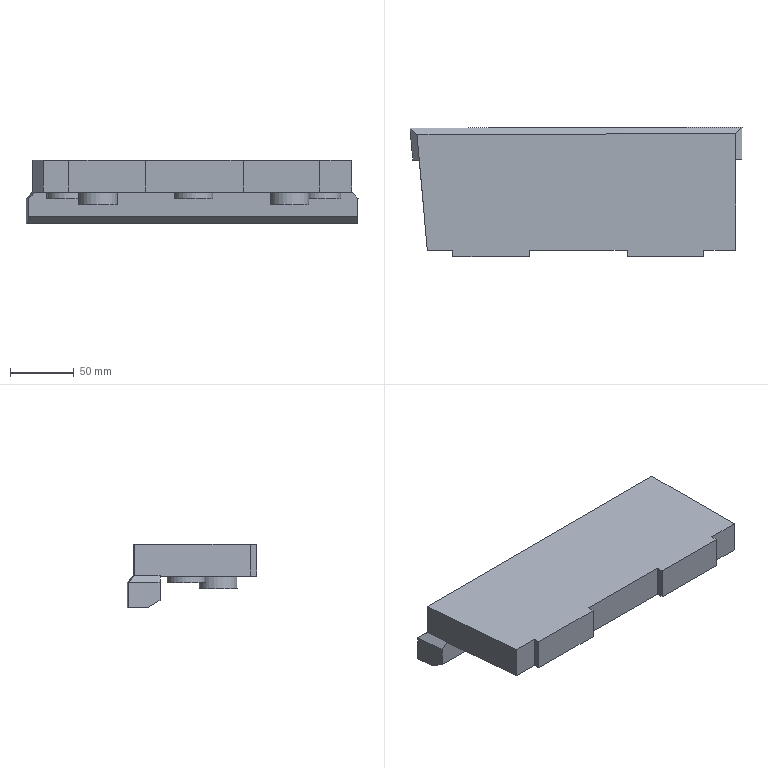Part | NX | features solid 2 | 1 solid | 33 faces | box 260.006 x 101.237 x 49.723 mm | volume 746762 mm3 | plane 22 | spline 6 | cylinder 5 | commonest cylinder face diameters 30 x5